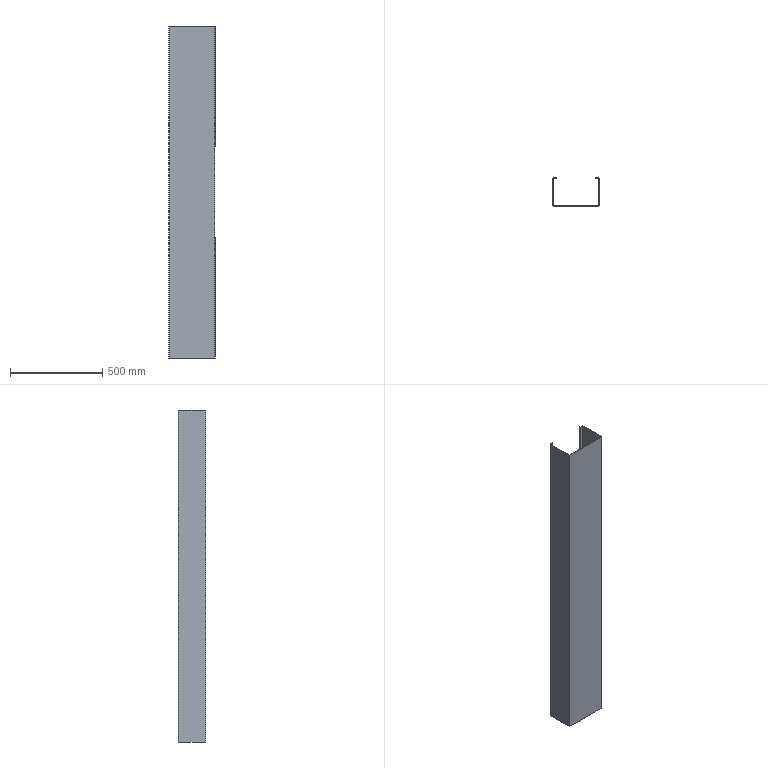Part | STEP file | 750038222 | 1 solid | 36 faces | box 250 x 150 x 1800 mm | volume 1443469 mm3 | plane 25 | cylinder 11 | commonest cylinder face diameters 3 x6 6 x5
STEP:
#1=CARTESIAN_POINT('',(124.598,1.5,248.5));
#2=VERTEX_POINT('',#1);
#3=CARTESIAN_POINT('',(122.,1.5,248.5));
#4=VERTEX_POINT('',#3);
#5=CARTESIAN_POINT('',(125.,1.5,248.5));
#6=DIRECTION('',(-1.,0.,0.));
#7=VECTOR('',#6,1000.);
#8=LINE('',#5,#7);
#9=EDGE_CURVE('',#2,#4,#8,.T.);
#10=ORIENTED_EDGE('',*,*,#9,.F.);
#11=CARTESIAN_POINT('',(124.598,1.5,-248.5));
#12=VERTEX_POINT('',#11);
#13=CARTESIAN_POINT('',(124.598,1.5,900.));
#14=DIRECTION('',(0.,0.,1.));
#15=VECTOR('',#14,1000.);
#16=LINE('',#13,#15);
#17=EDGE_CURVE('',#12,#2,#16,.T.);
#18=ORIENTED_EDGE('',*,*,#17,.F.);
#19=CARTESIAN_POINT('',(122.,1.5,-248.5));
#20=VERTEX_POINT('',#19);
#21=CARTESIAN_POINT('',(125.,1.5,-248.5));
#22=DIRECTION('',(1.,0.,0.));
#23=VECTOR('',#22,1000.);
#24=LINE('',#21,#23);
#25=EDGE_CURVE('',#20,#12,#24,.T.);
#26=ORIENTED_EDGE('',*,*,#25,.F.);
#27=CARTESIAN_POINT('',(122.,1.5,-900.));
#28=VERTEX_POINT('',#27);
#29=CARTESIAN_POINT('',(122.,1.5,900.));
#30=DIRECTION('',(0.,0.,1.));
#31=VECTOR('',#30,1000.);
#32=LINE('',#29,#31);
#33=EDGE_CURVE('',#28,#20,#32,.T.);
#34=ORIENTED_EDGE('',*,*,#33,.F.);
#35=CARTESIAN_POINT('',(-122.,1.5,-900.));
#36=VERTEX_POINT('',#35);
#37=CARTESIAN_POINT('',(125.,1.5,-900.));
#38=DIRECTION('',(1.,0.,0.));
#39=VECTOR('',#38,1000.);
#40=LINE('',#37,#39);
#41=EDGE_CURVE('',#36,#28,#40,.T.);
#42=ORIENTED_EDGE('',*,*,#41,.F.);
#43=CARTESIAN_POINT('',(-122.,1.5,900.));
#44=VERTEX_POINT('',#43);
#45=CARTESIAN_POINT('',(-122.,1.5,900.));
#46=DIRECTION('',(0.,0.,-1.));
#47=VECTOR('',#46,1000.);
#48=LINE('',#45,#47);
#49=EDGE_CURVE('',#44,#36,#48,.T.);
#50=ORIENTED_EDGE('',*,*,#49,.F.);
#51=CARTESIAN_POINT('',(122.,1.5,900.));
#52=VERTEX_POINT('',#51);
#53=CARTESIAN_POINT('',(125.,1.5,900.));
#54=DIRECTION('',(-1.,0.,0.));
#55=VECTOR('',#54,1000.);
#56=LINE('',#53,#55);
#57=EDGE_CURVE('',#52,#44,#56,.T.);
#58=ORIENTED_EDGE('',*,*,#57,.F.);
#59=CARTESIAN_POINT('',(122.,1.5,900.));
#60=DIRECTION('',(0.,0.,1.));
#61=VECTOR('',#60,1000.);
#62=LINE('',#59,#61);
#63=EDGE_CURVE('',#4,#52,#62,.T.);
#64=ORIENTED_EDGE('',*,*,#63,.F.);
#65=EDGE_LOOP('',(#10,#18,#26,#34,#42,#50,#58,#64));
#66=FACE_OUTER_BOUND('',#65,.T.);
#67=CARTESIAN_POINT('',(125.,1.5,900.));
#68=DIRECTION('',(0.,-1.,0.));
#69=DIRECTION('',(0.,0.,-1.));
#70=AXIS2_PLACEMENT_3D('',#67,#68,#69);
#71=PLANE('',#70);
#72=ADVANCED_FACE('',(#66),#71,.F.);
#73=CARTESIAN_POINT('',(123.5,3.,248.5));
#74=VERTEX_POINT('',#73);
#75=CARTESIAN_POINT('',(122.,3.,248.5));
#76=DIRECTION('',(0.,0.,1.));
#77=DIRECTION('',(-1.,0.,0.));
#78=AXIS2_PLACEMENT_3D('',#75,#76,#77);
#79=CIRCLE('',#78,1.5);
#80=EDGE_CURVE('',#4,#74,#79,.T.);
#81=ORIENTED_EDGE('',*,*,#80,.F.);
#82=ORIENTED_EDGE('',*,*,#63,.T.);
#83=CARTESIAN_POINT('',(123.5,3.,900.));
#84=VERTEX_POINT('',#83);
#85=CARTESIAN_POINT('',(122.,3.,900.));
#86=DIRECTION('',(0.,0.,-1.));
#87=DIRECTION('',(-1.,0.,0.));
#88=AXIS2_PLACEMENT_3D('',#85,#86,#87);
#89=CIRCLE('',#88,1.5);
#90=EDGE_CURVE('',#84,#52,#89,.T.);
#91=ORIENTED_EDGE('',*,*,#90,.F.);
#92=CARTESIAN_POINT('',(123.5,3.,900.));
#93=DIRECTION('',(0.,0.,1.));
#94=VECTOR('',#93,1000.);
#95=LINE('',#92,#94);
#96=EDGE_CURVE('',#74,#84,#95,.T.);
#97=ORIENTED_EDGE('',*,*,#96,.F.);
#98=EDGE_LOOP('',(#81,#82,#91,#97));
#99=FACE_OUTER_BOUND('',#98,.T.);
#100=CARTESIAN_POINT('',(122.,3.,900.));
#101=DIRECTION('',(0.,0.,-1.));
#102=DIRECTION('',(-1.,0.,0.));
#103=AXIS2_PLACEMENT_3D('',#100,#101,#102);
#104=CYLINDRICAL_SURFACE('',#103,1.5);
#105=ADVANCED_FACE('',(#99),#104,.F.);
#106=CARTESIAN_POINT('',(125.,147.,248.5));
#107=VERTEX_POINT('',#106);
#108=CARTESIAN_POINT('',(122.,150.,248.5));
#109=VERTEX_POINT('',#108);
#110=CARTESIAN_POINT('',(122.,147.,248.5));
#111=DIRECTION('',(0.,0.,1.));
#112=DIRECTION('',(-1.,0.,0.));
#113=AXIS2_PLACEMENT_3D('',#110,#111,#112);
#114=CIRCLE('',#113,3.);
#115=EDGE_CURVE('',#107,#109,#114,.T.);
#116=ORIENTED_EDGE('',*,*,#115,.F.);
#117=CARTESIAN_POINT('',(125.,3.,248.5));
#118=VERTEX_POINT('',#117);
#119=CARTESIAN_POINT('',(125.,1.5,248.5));
#120=DIRECTION('',(0.,1.,0.));
#121=VECTOR('',#120,1000.);
#122=LINE('',#119,#121);
#123=EDGE_CURVE('',#118,#107,#122,.T.);
#124=ORIENTED_EDGE('',*,*,#123,.F.);
#125=CARTESIAN_POINT('',(122.,3.,248.5));
#126=DIRECTION('',(0.,0.,1.));
#127=DIRECTION('',(-1.,0.,0.));
#128=AXIS2_PLACEMENT_3D('',#125,#126,#127);
#129=CIRCLE('',#128,3.);
#130=EDGE_CURVE('',#2,#118,#129,.T.);
#131=ORIENTED_EDGE('',*,*,#130,.F.);
#132=ORIENTED_EDGE('',*,*,#9,.T.);
#133=ORIENTED_EDGE('',*,*,#80,.T.);
#134=CARTESIAN_POINT('',(123.5,147.,248.5));
#135=VERTEX_POINT('',#134);
#136=CARTESIAN_POINT('',(123.5,1.5,248.5));
#137=DIRECTION('',(0.,-1.,0.));
#138=VECTOR('',#137,1000.);
#139=LINE('',#136,#138);
#140=EDGE_CURVE('',#135,#74,#139,.T.);
#141=ORIENTED_EDGE('',*,*,#140,.F.);
#142=CARTESIAN_POINT('',(122.,148.5,248.5));
#143=VERTEX_POINT('',#142);
#144=CARTESIAN_POINT('',(122.,147.,248.5));
#145=DIRECTION('',(0.,0.,-1.));
#146=DIRECTION('',(-1.,0.,0.));
#147=AXIS2_PLACEMENT_3D('',#144,#145,#146);
#148=CIRCLE('',#147,1.5);
#149=EDGE_CURVE('',#143,#135,#148,.T.);
#150=ORIENTED_EDGE('',*,*,#149,.F.);
#151=CARTESIAN_POINT('',(122.,148.5,248.5));
#152=DIRECTION('',(0.,1.,0.));
#153=VECTOR('',#152,1000.);
#154=LINE('',#151,#153);
#155=EDGE_CURVE('',#143,#109,#154,.T.);
#156=ORIENTED_EDGE('',*,*,#155,.T.);
#157=EDGE_LOOP('',(#116,#124,#131,#132,#133,#141,#150,#156));
#158=FACE_OUTER_BOUND('',#157,.T.);
#159=CARTESIAN_POINT('',(105.,1.5,248.5));
#160=DIRECTION('',(0.,0.,1.));
#161=DIRECTION('',(1.,0.,0.));
#162=AXIS2_PLACEMENT_3D('',#159,#160,#161);
#163=PLANE('',#162);
#164=ADVANCED_FACE('',(#158),#163,.F.);
#165=CARTESIAN_POINT('',(125.,3.,-248.5));
#166=VERTEX_POINT('',#165);
#167=CARTESIAN_POINT('',(122.,3.,-248.5));
#168=DIRECTION('',(0.,0.,-1.));
#169=DIRECTION('',(-1.,0.,0.));
#170=AXIS2_PLACEMENT_3D('',#167,#168,#169);
#171=CIRCLE('',#170,3.);
#172=EDGE_CURVE('',#166,#12,#171,.T.);
#173=ORIENTED_EDGE('',*,*,#172,.T.);
#174=ORIENTED_EDGE('',*,*,#17,.T.);
#175=ORIENTED_EDGE('',*,*,#130,.T.);
#176=CARTESIAN_POINT('',(125.,3.,900.));
#177=VERTEX_POINT('',#176);
#178=CARTESIAN_POINT('',(125.,3.,900.));
#179=DIRECTION('',(0.,0.,1.));
#180=VECTOR('',#179,1000.);
#181=LINE('',#178,#180);
#182=EDGE_CURVE('',#118,#177,#181,.T.);
#183=ORIENTED_EDGE('',*,*,#182,.T.);
#184=CARTESIAN_POINT('',(122.,0.,900.));
#185=VERTEX_POINT('',#184);
#186=CARTESIAN_POINT('',(122.,3.,900.));
#187=DIRECTION('',(0.,0.,-1.));
#188=DIRECTION('',(-1.,0.,0.));
#189=AXIS2_PLACEMENT_3D('',#186,#187,#188);
#190=CIRCLE('',#189,3.);
#191=EDGE_CURVE('',#177,#185,#190,.T.);
#192=ORIENTED_EDGE('',*,*,#191,.T.);
#193=CARTESIAN_POINT('',(122.,0.,-900.));
#194=VERTEX_POINT('',#193);
#195=CARTESIAN_POINT('',(122.,0.,900.));
#196=DIRECTION('',(0.,0.,-1.));
#197=VECTOR('',#196,1000.);
#198=LINE('',#195,#197);
#199=EDGE_CURVE('',#185,#194,#198,.T.);
#200=ORIENTED_EDGE('',*,*,#199,.T.);
#201=CARTESIAN_POINT('',(125.,3.,-900.));
#202=VERTEX_POINT('',#201);
#203=CARTESIAN_POINT('',(122.,3.,-900.));
#204=DIRECTION('',(0.,0.,1.));
#205=DIRECTION('',(-1.,0.,0.));
#206=AXIS2_PLACEMENT_3D('',#203,#204,#205);
#207=CIRCLE('',#206,3.);
#208=EDGE_CURVE('',#194,#202,#207,.T.);
#209=ORIENTED_EDGE('',*,*,#208,.T.);
#210=CARTESIAN_POINT('',(125.,3.,900.));
#211=DIRECTION('',(0.,0.,1.));
#212=VECTOR('',#211,1000.);
#213=LINE('',#210,#212);
#214=EDGE_CURVE('',#202,#166,#213,.T.);
#215=ORIENTED_EDGE('',*,*,#214,.T.);
#216=EDGE_LOOP('',(#173,#174,#175,#183,#192,#200,#209,#215));
#217=FACE_OUTER_BOUND('',#216,.T.);
#218=CARTESIAN_POINT('',(122.,3.,900.));
#219=DIRECTION('',(0.,0.,-1.));
#220=DIRECTION('',(-1.,0.,0.));
#221=AXIS2_PLACEMENT_3D('',#218,#219,#220);
#222=CYLINDRICAL_SURFACE('',#221,3.);
#223=ADVANCED_FACE('',(#217),#222,.T.);
#224=CARTESIAN_POINT('',(122.,148.5,-248.5));
#225=VERTEX_POINT('',#224);
#226=CARTESIAN_POINT('',(122.,150.,-248.5));
#227=VERTEX_POINT('',#226);
#228=CARTESIAN_POINT('',(122.,148.5,-248.5));
#229=DIRECTION('',(0.,1.,0.));
#230=VECTOR('',#229,1000.);
#231=LINE('',#228,#230);
#232=EDGE_CURVE('',#225,#227,#231,.T.);
#233=ORIENTED_EDGE('',*,*,#232,.F.);
#234=CARTESIAN_POINT('',(123.5,147.,-248.5));
#235=VERTEX_POINT('',#234);
#236=CARTESIAN_POINT('',(122.,147.,-248.5));
#237=DIRECTION('',(0.,0.,1.));
#238=DIRECTION('',(-1.,0.,0.));
#239=AXIS2_PLACEMENT_3D('',#236,#237,#238);
#240=CIRCLE('',#239,1.5);
#241=EDGE_CURVE('',#235,#225,#240,.T.);
#242=ORIENTED_EDGE('',*,*,#241,.F.);
#243=CARTESIAN_POINT('',(123.5,3.,-248.5));
#244=VERTEX_POINT('',#243);
#245=CARTESIAN_POINT('',(123.5,1.5,-248.5));
#246=DIRECTION('',(0.,1.,0.));
#247=VECTOR('',#246,1000.);
#248=LINE('',#245,#247);
#249=EDGE_CURVE('',#244,#235,#248,.T.);
#250=ORIENTED_EDGE('',*,*,#249,.F.);
#251=CARTESIAN_POINT('',(122.,3.,-248.5));
#252=DIRECTION('',(0.,0.,1.));
#253=DIRECTION('',(-1.,0.,0.));
#254=AXIS2_PLACEMENT_3D('',#251,#252,#253);
#255=CIRCLE('',#254,1.5);
#256=EDGE_CURVE('',#20,#244,#255,.T.);
#257=ORIENTED_EDGE('',*,*,#256,.F.);
#258=ORIENTED_EDGE('',*,*,#25,.T.);
#259=ORIENTED_EDGE('',*,*,#172,.F.);
#260=CARTESIAN_POINT('',(125.,147.,-248.5));
#261=VERTEX_POINT('',#260);
#262=CARTESIAN_POINT('',(125.,1.5,-248.5));
#263=DIRECTION('',(0.,-1.,0.));
#264=VECTOR('',#263,1000.);
#265=LINE('',#262,#264);
#266=EDGE_CURVE('',#261,#166,#265,.T.);
#267=ORIENTED_EDGE('',*,*,#266,.F.);
#268=CARTESIAN_POINT('',(122.,147.,-248.5));
#269=DIRECTION('',(0.,0.,-1.));
#270=DIRECTION('',(-1.,0.,0.));
#271=AXIS2_PLACEMENT_3D('',#268,#269,#270);
#272=CIRCLE('',#271,3.);
#273=EDGE_CURVE('',#227,#261,#272,.T.);
#274=ORIENTED_EDGE('',*,*,#273,.F.);
#275=EDGE_LOOP('',(#233,#242,#250,#257,#258,#259,#267,#274));
#276=FACE_OUTER_BOUND('',#275,.T.);
#277=CARTESIAN_POINT('',(125.,1.5,-248.5));
#278=DIRECTION('',(0.,0.,-1.));
#279=DIRECTION('',(-1.,0.,0.));
#280=AXIS2_PLACEMENT_3D('',#277,#278,#279);
#281=PLANE('',#280);
#282=ADVANCED_FACE('',(#276),#281,.F.);
#283=ORIENTED_EDGE('',*,*,#256,.T.);
#284=CARTESIAN_POINT('',(123.5,3.,-900.));
#285=VERTEX_POINT('',#284);
#286=CARTESIAN_POINT('',(123.5,3.,900.));
#287=DIRECTION('',(0.,0.,1.));
#288=VECTOR('',#287,1000.);
#289=LINE('',#286,#288);
#290=EDGE_CURVE('',#285,#244,#289,.T.);
#291=ORIENTED_EDGE('',*,*,#290,.F.);
#292=CARTESIAN_POINT('',(122.,3.,-900.));
#293=DIRECTION('',(0.,0.,1.));
#294=DIRECTION('',(-1.,0.,0.));
#295=AXIS2_PLACEMENT_3D('',#292,#293,#294);
#296=CIRCLE('',#295,1.5);
#297=EDGE_CURVE('',#28,#285,#296,.T.);
#298=ORIENTED_EDGE('',*,*,#297,.F.);
#299=ORIENTED_EDGE('',*,*,#33,.T.);
#300=EDGE_LOOP('',(#283,#291,#298,#299));
#301=FACE_OUTER_BOUND('',#300,.T.);
#302=CARTESIAN_POINT('',(122.,3.,900.));
#303=DIRECTION('',(0.,0.,-1.));
#304=DIRECTION('',(-1.,0.,0.));
#305=AXIS2_PLACEMENT_3D('',#302,#303,#304);
#306=CYLINDRICAL_SURFACE('',#305,1.5);
#307=ADVANCED_FACE('',(#301),#306,.F.);
#308=CARTESIAN_POINT('',(105.,148.5,-900.));
#309=VERTEX_POINT('',#308);
#310=CARTESIAN_POINT('',(122.,148.5,-900.));
#311=VERTEX_POINT('',#310);
#312=CARTESIAN_POINT('',(105.,148.5,-900.));
#313=DIRECTION('',(1.,0.,0.));
#314=VECTOR('',#313,1000.);
#315=LINE('',#312,#314);
#316=EDGE_CURVE('',#309,#311,#315,.T.);
#317=ORIENTED_EDGE('',*,*,#316,.F.);
#318=CARTESIAN_POINT('',(105.,150.,-900.));
#319=VERTEX_POINT('',#318);
#320=CARTESIAN_POINT('',(105.,150.,-900.));
#321=DIRECTION('',(0.,1.,0.));
#322=VECTOR('',#321,1000.);
#323=LINE('',#320,#322);
#324=EDGE_CURVE('',#309,#319,#323,.T.);
#325=ORIENTED_EDGE('',*,*,#324,.T.);
#326=CARTESIAN_POINT('',(122.,150.,-900.));
#327=VERTEX_POINT('',#326);
#328=CARTESIAN_POINT('',(105.,150.,-900.));
#329=DIRECTION('',(-1.,0.,0.));
#330=VECTOR('',#329,1000.);
#331=LINE('',#328,#330);
#332=EDGE_CURVE('',#327,#319,#331,.T.);
#333=ORIENTED_EDGE('',*,*,#332,.F.);
#334=CARTESIAN_POINT('',(125.,147.,-900.));
#335=VERTEX_POINT('',#334);
#336=CARTESIAN_POINT('',(122.,147.,-900.));
#337=DIRECTION('',(0.,0.,1.));
#338=DIRECTION('',(-1.,0.,0.));
#339=AXIS2_PLACEMENT_3D('',#336,#337,#338);
#340=CIRCLE('',#339,3.);
#341=EDGE_CURVE('',#335,#327,#340,.T.);
#342=ORIENTED_EDGE('',*,*,#341,.F.);
#343=CARTESIAN_POINT('',(125.,150.,-900.));
#344=DIRECTION('',(0.,1.,0.));
#345=VECTOR('',#344,1000.);
#346=LINE('',#343,#345);
#347=EDGE_CURVE('',#202,#335,#346,.T.);
#348=ORIENTED_EDGE('',*,*,#347,.F.);
#349=ORIENTED_EDGE('',*,*,#208,.F.);
#350=CARTESIAN_POINT('',(-122.,0.,-900.));
#351=VERTEX_POINT('',#350);
#352=CARTESIAN_POINT('',(105.,0.,-900.));
#353=DIRECTION('',(1.,0.,0.));
#354=VECTOR('',#353,1000.);
#355=LINE('',#352,#354);
#356=EDGE_CURVE('',#351,#194,#355,.T.);
#357=ORIENTED_EDGE('',*,*,#356,.F.);
#358=CARTESIAN_POINT('',(-125.,3.,-900.));
#359=VERTEX_POINT('',#358);
#360=CARTESIAN_POINT('',(-122.,3.,-900.));
#361=DIRECTION('',(0.,0.,1.));
#362=DIRECTION('',(-1.,0.,0.));
#363=AXIS2_PLACEMENT_3D('',#360,#361,#362);
#364=CIRCLE('',#363,3.);
#365=EDGE_CURVE('',#359,#351,#364,.T.);
#366=ORIENTED_EDGE('',*,*,#365,.F.);
#367=CARTESIAN_POINT('',(-125.,147.,-900.));
#368=VERTEX_POINT('',#367);
#369=CARTESIAN_POINT('',(-125.,150.,-900.));
#370=DIRECTION('',(0.,-1.,0.));
#371=VECTOR('',#370,1000.);
#372=LINE('',#369,#371);
#373=EDGE_CURVE('',#368,#359,#372,.T.);
#374=ORIENTED_EDGE('',*,*,#373,.F.);
#375=CARTESIAN_POINT('',(-122.,150.,-900.));
#376=VERTEX_POINT('',#375);
#377=CARTESIAN_POINT('',(-122.,147.,-900.));
#378=DIRECTION('',(0.,0.,1.));
#379=DIRECTION('',(-1.,0.,0.));
#380=AXIS2_PLACEMENT_3D('',#377,#378,#379);
#381=CIRCLE('',#380,3.);
#382=EDGE_CURVE('',#376,#368,#381,.T.);
#383=ORIENTED_EDGE('',*,*,#382,.F.);
#384=CARTESIAN_POINT('',(-105.,150.,-900.));
#385=VERTEX_POINT('',#384);
#386=CARTESIAN_POINT('',(105.,150.,-900.));
#387=DIRECTION('',(-1.,0.,0.));
#388=VECTOR('',#387,1000.);
#389=LINE('',#386,#388);
#390=EDGE_CURVE('',#385,#376,#389,.T.);
#391=ORIENTED_EDGE('',*,*,#390,.F.);
#392=CARTESIAN_POINT('',(-105.,148.5,-900.));
#393=VERTEX_POINT('',#392);
#394=CARTESIAN_POINT('',(-105.,150.,-900.));
#395=DIRECTION('',(0.,1.,0.));
#396=VECTOR('',#395,1000.);
#397=LINE('',#394,#396);
#398=EDGE_CURVE('',#393,#385,#397,.T.);
#399=ORIENTED_EDGE('',*,*,#398,.F.);
#400=CARTESIAN_POINT('',(-122.,148.5,-900.));
#401=VERTEX_POINT('',#400);
#402=CARTESIAN_POINT('',(105.,148.5,-900.));
#403=DIRECTION('',(1.,0.,0.));
#404=VECTOR('',#403,1000.);
#405=LINE('',#402,#404);
#406=EDGE_CURVE('',#401,#393,#405,.T.);
#407=ORIENTED_EDGE('',*,*,#406,.F.);
#408=CARTESIAN_POINT('',(-123.5,147.,-900.));
#409=VERTEX_POINT('',#408);
#410=CARTESIAN_POINT('',(-122.,147.,-900.));
#411=DIRECTION('',(0.,0.,-1.));
#412=DIRECTION('',(-1.,0.,0.));
#413=AXIS2_PLACEMENT_3D('',#410,#411,#412);
#414=CIRCLE('',#413,1.5);
#415=EDGE_CURVE('',#409,#401,#414,.T.);
#416=ORIENTED_EDGE('',*,*,#415,.F.);
#417=CARTESIAN_POINT('',(-123.5,3.,-900.));
#418=VERTEX_POINT('',#417);
#419=CARTESIAN_POINT('',(-123.5,150.,-900.));
#420=DIRECTION('',(0.,1.,0.));
#421=VECTOR('',#420,1000.);
#422=LINE('',#419,#421);
#423=EDGE_CURVE('',#418,#409,#422,.T.);
#424=ORIENTED_EDGE('',*,*,#423,.F.);
#425=CARTESIAN_POINT('',(-122.,3.,-900.));
#426=DIRECTION('',(0.,0.,-1.));
#427=DIRECTION('',(-1.,0.,0.));
#428=AXIS2_PLACEMENT_3D('',#425,#426,#427);
#429=CIRCLE('',#428,1.5);
#430=EDGE_CURVE('',#36,#418,#429,.T.);
#431=ORIENTED_EDGE('',*,*,#430,.F.);
#432=ORIENTED_EDGE('',*,*,#41,.T.);
#433=ORIENTED_EDGE('',*,*,#297,.T.);
#434=CARTESIAN_POINT('',(123.5,147.,-900.));
#435=VERTEX_POINT('',#434);
#436=CARTESIAN_POINT('',(123.5,150.,-900.));
#437=DIRECTION('',(0.,-1.,0.));
#438=VECTOR('',#437,1000.);
#439=LINE('',#436,#438);
#440=EDGE_CURVE('',#435,#285,#439,.T.);
#441=ORIENTED_EDGE('',*,*,#440,.F.);
#442=CARTESIAN_POINT('',(122.,147.,-900.));
#443=DIRECTION('',(0.,0.,-1.));
#444=DIRECTION('',(-1.,0.,0.));
#445=AXIS2_PLACEMENT_3D('',#442,#443,#444);
#446=CIRCLE('',#445,1.5);
#447=EDGE_CURVE('',#311,#435,#446,.T.);
#448=ORIENTED_EDGE('',*,*,#447,.F.);
#449=EDGE_LOOP('',(#317,#325,#333,#342,#348,#349,#357,#366,#374,#383,#391,#399,#407,#416,#424,#431,#432,#433,#441,#448));
#450=FACE_OUTER_BOUND('',#449,.T.);
#451=CARTESIAN_POINT('',(105.,150.,-900.));
#452=DIRECTION('',(0.,0.,1.));
#453=DIRECTION('',(1.,0.,0.));
#454=AXIS2_PLACEMENT_3D('',#451,#452,#453);
#455=PLANE('',#454);
#456=ADVANCED_FACE('',(#450),#455,.F.);
#457=CARTESIAN_POINT('',(-123.5,3.,900.));
#458=VERTEX_POINT('',#457);
#459=CARTESIAN_POINT('',(-123.5,3.,900.));
#460=DIRECTION('',(0.,0.,-1.));
#461=VECTOR('',#460,1000.);
#462=LINE('',#459,#461);
#463=EDGE_CURVE('',#458,#418,#462,.T.);
#464=ORIENTED_EDGE('',*,*,#463,.F.);
#465=CARTESIAN_POINT('',(-122.,3.,900.));
#466=DIRECTION('',(0.,0.,-1.));
#467=DIRECTION('',(-1.,0.,0.));
#468=AXIS2_PLACEMENT_3D('',#465,#466,#467);
#469=CIRCLE('',#468,1.5);
#470=EDGE_CURVE('',#44,#458,#469,.T.);
#471=ORIENTED_EDGE('',*,*,#470,.F.);
#472=ORIENTED_EDGE('',*,*,#49,.T.);
#473=ORIENTED_EDGE('',*,*,#430,.T.);
#474=EDGE_LOOP('',(#464,#471,#472,#473));
#475=FACE_OUTER_BOUND('',#474,.T.);
#476=CARTESIAN_POINT('',(-122.,3.,900.));
#477=DIRECTION('',(0.,0.,-1.));
#478=DIRECTION('',(-1.,0.,0.));
#479=AXIS2_PLACEMENT_3D('',#476,#477,#478);
#480=CYLINDRICAL_SURFACE('',#479,1.5);
#481=ADVANCED_FACE('',(#475),#480,.F.);
#482=CARTESIAN_POINT('',(-122.,148.5,900.));
#483=VERTEX_POINT('',#482);
#484=CARTESIAN_POINT('',(-105.,148.5,900.));
#485=VERTEX_POINT('',#484);
#486=CARTESIAN_POINT('',(-125.,148.5,900.));
#487=DIRECTION('',(1.,0.,0.));
#488=VECTOR('',#487,1000.);
#489=LINE('',#486,#488);
#490=EDGE_CURVE('',#483,#485,#489,.T.);
#491=ORIENTED_EDGE('',*,*,#490,.T.);
#492=CARTESIAN_POINT('',(-105.,150.,900.));
#493=VERTEX_POINT('',#492);
#494=CARTESIAN_POINT('',(-105.,150.,900.));
#495=DIRECTION('',(0.,-1.,0.));
#496=VECTOR('',#495,1000.);
#497=LINE('',#494,#496);
#498=EDGE_CURVE('',#493,#485,#497,.T.);
#499=ORIENTED_EDGE('',*,*,#498,.F.);
#500=CARTESIAN_POINT('',(-122.,150.,900.));
#501=VERTEX_POINT('',#500);
#502=CARTESIAN_POINT('',(-125.,150.,900.));
#503=DIRECTION('',(-1.,0.,0.));
#504=VECTOR('',#503,1000.);
#505=LINE('',#502,#504);
#506=EDGE_CURVE('',#493,#501,#505,.T.);
#507=ORIENTED_EDGE('',*,*,#506,.T.);
#508=CARTESIAN_POINT('',(-125.,147.,900.));
#509=VERTEX_POINT('',#508);
#510=CARTESIAN_POINT('',(-122.,147.,900.));
#511=DIRECTION('',(0.,0.,1.));
#512=DIRECTION('',(-1.,0.,0.));
#513=AXIS2_PLACEMENT_3D('',#510,#511,#512);
#514=CIRCLE('',#513,3.);
#515=EDGE_CURVE('',#501,#509,#514,.T.);
#516=ORIENTED_EDGE('',*,*,#515,.T.);
#517=CARTESIAN_POINT('',(-125.,3.,900.));
#518=VERTEX_POINT('',#517);
#519=CARTESIAN_POINT('',(-125.,150.,900.));
#520=DIRECTION('',(0.,-1.,0.));
#521=VECTOR('',#520,1000.);
#522=LINE('',#519,#521);
#523=EDGE_CURVE('',#509,#518,#522,.T.);
#524=ORIENTED_EDGE('',*,*,#523,.T.);
#525=CARTESIAN_POINT('',(-122.,0.,900.));
#526=VERTEX_POINT('',#525);
#527=CARTESIAN_POINT('',(-122.,3.,900.));
#528=DIRECTION('',(0.,0.,1.));
#529=DIRECTION('',(-1.,0.,0.));
#530=AXIS2_PLACEMENT_3D('',#527,#528,#529);
#531=CIRCLE('',#530,3.);
#532=EDGE_CURVE('',#518,#526,#531,.T.);
#533=ORIENTED_EDGE('',*,*,#532,.T.);
#534=CARTESIAN_POINT('',(-125.,0.,900.));
#535=DIRECTION('',(1.,0.,0.));
#536=VECTOR('',#535,1000.);
#537=LINE('',#534,#536);
#538=EDGE_CURVE('',#526,#185,#537,.T.);
#539=ORIENTED_EDGE('',*,*,#538,.T.);
#540=ORIENTED_EDGE('',*,*,#191,.F.);
#541=CARTESIAN_POINT('',(125.,147.,900.));
#542=VERTEX_POINT('',#541);
#543=CARTESIAN_POINT('',(125.,150.,900.));
#544=DIRECTION('',(0.,1.,0.));
#545=VECTOR('',#544,1000.);
#546=LINE('',#543,#545);
#547=EDGE_CURVE('',#177,#542,#546,.T.);
#548=ORIENTED_EDGE('',*,*,#547,.T.);
#549=CARTESIAN_POINT('',(122.,150.,900.));
#550=VERTEX_POINT('',#549);
#551=CARTESIAN_POINT('',(122.,147.,900.));
#552=DIRECTION('',(0.,0.,1.));
#553=DIRECTION('',(-1.,0.,0.));
#554=AXIS2_PLACEMENT_3D('',#551,#552,#553);
#555=CIRCLE('',#554,3.);
#556=EDGE_CURVE('',#542,#550,#555,.T.);
#557=ORIENTED_EDGE('',*,*,#556,.T.);
#558=CARTESIAN_POINT('',(105.,150.,900.));
#559=VERTEX_POINT('',#558);
#560=CARTESIAN_POINT('',(-125.,150.,900.));
#561=DIRECTION('',(-1.,0.,0.));
#562=VECTOR('',#561,1000.);
#563=LINE('',#560,#562);
#564=EDGE_CURVE('',#550,#559,#563,.T.);
#565=ORIENTED_EDGE('',*,*,#564,.T.);
#566=CARTESIAN_POINT('',(105.,148.5,900.));
#567=VERTEX_POINT('',#566);
#568=CARTESIAN_POINT('',(105.,150.,900.));
#569=DIRECTION('',(0.,-1.,0.));
#570=VECTOR('',#569,1000.);
#571=LINE('',#568,#570);
#572=EDGE_CURVE('',#559,#567,#571,.T.);
#573=ORIENTED_EDGE('',*,*,#572,.T.);
#574=CARTESIAN_POINT('',(122.,148.5,900.));
#575=VERTEX_POINT('',#574);
#576=CARTESIAN_POINT('',(-125.,148.5,900.));
#577=DIRECTION('',(1.,0.,0.));
#578=VECTOR('',#577,1000.);
#579=LINE('',#576,#578);
#580=EDGE_CURVE('',#567,#575,#579,.T.);
#581=ORIENTED_EDGE('',*,*,#580,.T.);
#582=CARTESIAN_POINT('',(123.5,147.,900.));
#583=VERTEX_POINT('',#582);
#584=CARTESIAN_POINT('',(122.,147.,900.));
#585=DIRECTION('',(0.,0.,-1.));
#586=DIRECTION('',(-1.,0.,0.));
#587=AXIS2_PLACEMENT_3D('',#584,#585,#586);
#588=CIRCLE('',#587,1.5);
#589=EDGE_CURVE('',#575,#583,#588,.T.);
#590=ORIENTED_EDGE('',*,*,#589,.T.);
#591=CARTESIAN_POINT('',(123.5,150.,900.));
#592=DIRECTION('',(0.,-1.,0.));
#593=VECTOR('',#592,1000.);
#594=LINE('',#591,#593);
#595=EDGE_CURVE('',#583,#84,#594,.T.);
#596=ORIENTED_EDGE('',*,*,#595,.T.);
#597=ORIENTED_EDGE('',*,*,#90,.T.);
#598=ORIENTED_EDGE('',*,*,#57,.T.);
#599=ORIENTED_EDGE('',*,*,#470,.T.);
#600=CARTESIAN_POINT('',(-123.5,147.,900.));
#601=VERTEX_POINT('',#600);
#602=CARTESIAN_POINT('',(-123.5,150.,900.));
#603=DIRECTION('',(0.,1.,0.));
#604=VECTOR('',#603,1000.);
#605=LINE('',#602,#604);
#606=EDGE_CURVE('',#458,#601,#605,.T.);
#607=ORIENTED_EDGE('',*,*,#606,.T.);
#608=CARTESIAN_POINT('',(-122.,147.,900.));
#609=DIRECTION('',(0.,0.,-1.));
#610=DIRECTION('',(-1.,0.,0.));
#611=AXIS2_PLACEMENT_3D('',#608,#609,#610);
#612=CIRCLE('',#611,1.5);
#613=EDGE_CURVE('',#601,#483,#612,.T.);
#614=ORIENTED_EDGE('',*,*,#613,.T.);
#615=EDGE_LOOP('',(#491,#499,#507,#516,#524,#533,#539,#540,#548,#557,#565,#573,#581,#590,#596,#597,#598,#599,#607,#614));
#616=FACE_OUTER_BOUND('',#615,.T.);
#617=CARTESIAN_POINT('',(-125.,150.,900.));
#618=DIRECTION('',(0.,0.,1.));
#619=DIRECTION('',(1.,0.,0.));
#620=AXIS2_PLACEMENT_3D('',#617,#618,#619);
#621=PLANE('',#620);
#622=ADVANCED_FACE('',(#616),#621,.T.);
#623=ORIENTED_EDGE('',*,*,#140,.T.);
#624=ORIENTED_EDGE('',*,*,#96,.T.);
#625=ORIENTED_EDGE('',*,*,#595,.F.);
#626=CARTESIAN_POINT('',(123.5,147.,900.));
#627=DIRECTION('',(0.,0.,1.));
#628=VECTOR('',#627,1000.);
#629=LINE('',#626,#628);
#630=EDGE_CURVE('',#135,#583,#629,.T.);
#631=ORIENTED_EDGE('',*,*,#630,.F.);
#632=EDGE_LOOP('',(#623,#624,#625,#631));
#633=FACE_OUTER_BOUND('',#632,.T.);
#634=CARTESIAN_POINT('',(123.5,150.,900.));
#635=DIRECTION('',(1.,0.,0.));
#636=DIRECTION('',(0.,0.,-1.));
#637=AXIS2_PLACEMENT_3D('',#634,#635,#636);
#638=PLANE('',#637);
#639=ADVANCED_FACE('',(#633),#638,.F.);
#640=ORIENTED_EDGE('',*,*,#556,.F.);
#641=CARTESIAN_POINT('',(125.,147.,900.));
#642=DIRECTION('',(0.,0.,-1.));
#643=VECTOR('',#642,1000.);
#644=LINE('',#641,#643);
#645=EDGE_CURVE('',#542,#107,#644,.T.);
#646=ORIENTED_EDGE('',*,*,#645,.T.);
#647=ORIENTED_EDGE('',*,*,#115,.T.);
#648=CARTESIAN_POINT('',(122.,150.,900.));
#649=DIRECTION('',(0.,0.,1.));
#650=VECTOR('',#649,1000.);
#651=LINE('',#648,#650);
#652=EDGE_CURVE('',#109,#550,#651,.T.);
#653=ORIENTED_EDGE('',*,*,#652,.T.);
#654=EDGE_LOOP('',(#640,#646,#647,#653));
#655=FACE_OUTER_BOUND('',#654,.T.);
#656=CARTESIAN_POINT('',(122.,147.,900.));
#657=DIRECTION('',(0.,0.,-1.));
#658=DIRECTION('',(-1.,0.,0.));
#659=AXIS2_PLACEMENT_3D('',#656,#657,#658);
#660=CYLINDRICAL_SURFACE('',#659,3.);
#661=ADVANCED_FACE('',(#655),#660,.T.);
#662=ORIENTED_EDGE('',*,*,#645,.F.);
#663=ORIENTED_EDGE('',*,*,#547,.F.);
#664=ORIENTED_EDGE('',*,*,#182,.F.);
#665=ORIENTED_EDGE('',*,*,#123,.T.);
#666=EDGE_LOOP('',(#662,#663,#664,#665));
#667=FACE_OUTER_BOUND('',#666,.T.);
#668=CARTESIAN_POINT('',(125.,150.,900.));
#669=DIRECTION('',(1.,0.,0.));
#670=DIRECTION('',(0.,0.,-1.));
#671=AXIS2_PLACEMENT_3D('',#668,#669,#670);
#672=PLANE('',#671);
#673=ADVANCED_FACE('',(#667),#672,.T.);
#674=ORIENTED_EDGE('',*,*,#149,.T.);
#675=ORIENTED_EDGE('',*,*,#630,.T.);
#676=ORIENTED_EDGE('',*,*,#589,.F.);
#677=CARTESIAN_POINT('',(122.,148.5,900.));
#678=DIRECTION('',(0.,0.,1.));
#679=VECTOR('',#678,1000.);
#680=LINE('',#677,#679);
#681=EDGE_CURVE('',#143,#575,#680,.T.);
#682=ORIENTED_EDGE('',*,*,#681,.F.);
#683=EDGE_LOOP('',(#674,#675,#676,#682));
#684=FACE_OUTER_BOUND('',#683,.T.);
#685=CARTESIAN_POINT('',(122.,147.,900.));
#686=DIRECTION('',(0.,0.,-1.));
#687=DIRECTION('',(-1.,0.,0.));
#688=AXIS2_PLACEMENT_3D('',#685,#686,#687);
#689=CYLINDRICAL_SURFACE('',#688,1.5);
#690=ADVANCED_FACE('',(#684),#689,.F.);
#691=ORIENTED_EDGE('',*,*,#347,.T.);
#692=CARTESIAN_POINT('',(125.,147.,900.));
#693=DIRECTION('',(0.,0.,1.));
#694=VECTOR('',#693,1000.);
#695=LINE('',#692,#694);
#696=EDGE_CURVE('',#335,#261,#695,.T.);
#697=ORIENTED_EDGE('',*,*,#696,.T.);
#698=ORIENTED_EDGE('',*,*,#266,.T.);
#699=ORIENTED_EDGE('',*,*,#214,.F.);
#700=EDGE_LOOP('',(#691,#697,#698,#699));
#701=FACE_OUTER_BOUND('',#700,.T.);
#702=CARTESIAN_POINT('',(125.,150.,900.));
#703=DIRECTION('',(1.,0.,0.));
#704=DIRECTION('',(0.,0.,-1.));
#705=AXIS2_PLACEMENT_3D('',#702,#703,#704);
#706=PLANE('',#705);
#707=ADVANCED_FACE('',(#701),#706,.T.);
#708=ORIENTED_EDGE('',*,*,#538,.F.);
#709=CARTESIAN_POINT('',(-122.,0.,900.));
#710=DIRECTION('',(0.,0.,-1.));
#711=VECTOR('',#710,1000.);
#712=LINE('',#709,#711);
#713=EDGE_CURVE('',#526,#351,#712,.T.);
#714=ORIENTED_EDGE('',*,*,#713,.T.);
#715=ORIENTED_EDGE('',*,*,#356,.T.);
#716=ORIENTED_EDGE('',*,*,#199,.F.);
#717=EDGE_LOOP('',(#708,#714,#715,#716));
#718=FACE_OUTER_BOUND('',#717,.T.);
#719=CARTESIAN_POINT('',(125.,0.,900.));
#720=DIRECTION('',(0.,-1.,0.));
#721=DIRECTION('',(0.,0.,-1.));
#722=AXIS2_PLACEMENT_3D('',#719,#720,#721);
#723=PLANE('',#722);
#724=ADVANCED_FACE('',(#718),#723,.T.);
#725=ORIENTED_EDGE('',*,*,#341,.T.);
#726=CARTESIAN_POINT('',(122.,150.,900.));
#727=DIRECTION('',(0.,0.,1.));
#728=VECTOR('',#727,1000.);
#729=LINE('',#726,#728);
#730=EDGE_CURVE('',#327,#227,#729,.T.);
#731=ORIENTED_EDGE('',*,*,#730,.T.);
#732=ORIENTED_EDGE('',*,*,#273,.T.);
#733=ORIENTED_EDGE('',*,*,#696,.F.);
#734=EDGE_LOOP('',(#725,#731,#732,#733));
#735=FACE_OUTER_BOUND('',#734,.T.);
#736=CARTESIAN_POINT('',(122.,147.,900.));
#737=DIRECTION('',(0.,0.,-1.));
#738=DIRECTION('',(-1.,0.,0.));
#739=AXIS2_PLACEMENT_3D('',#736,#737,#738);
#740=CYLINDRICAL_SURFACE('',#739,3.);
#741=ADVANCED_FACE('',(#735),#740,.T.);
#742=ORIENTED_EDGE('',*,*,#241,.T.);
#743=CARTESIAN_POINT('',(122.,148.5,900.));
#744=DIRECTION('',(0.,0.,1.));
#745=VECTOR('',#744,1000.);
#746=LINE('',#743,#745);
#747=EDGE_CURVE('',#311,#225,#746,.T.);
#748=ORIENTED_EDGE('',*,*,#747,.F.);
#749=ORIENTED_EDGE('',*,*,#447,.T.);
#750=CARTESIAN_POINT('',(123.5,147.,900.));
#751=DIRECTION('',(0.,0.,-1.));
#752=VECTOR('',#751,1000.);
#753=LINE('',#750,#752);
#754=EDGE_CURVE('',#235,#435,#753,.T.);
#755=ORIENTED_EDGE('',*,*,#754,.F.);
#756=EDGE_LOOP('',(#742,#748,#749,#755));
#757=FACE_OUTER_BOUND('',#756,.T.);
#758=CARTESIAN_POINT('',(122.,147.,900.));
#759=DIRECTION('',(0.,0.,-1.));
#760=DIRECTION('',(-1.,0.,0.));
#761=AXIS2_PLACEMENT_3D('',#758,#759,#760);
#762=CYLINDRICAL_SURFACE('',#761,1.5);
#763=ADVANCED_FACE('',(#757),#762,.F.);
#764=ORIENTED_EDGE('',*,*,#249,.T.);
#765=ORIENTED_EDGE('',*,*,#754,.T.);
#766=ORIENTED_EDGE('',*,*,#440,.T.);
#767=ORIENTED_EDGE('',*,*,#290,.T.);
#768=EDGE_LOOP('',(#764,#765,#766,#767));
#769=FACE_OUTER_BOUND('',#768,.T.);
#770=CARTESIAN_POINT('',(123.5,150.,900.));
#771=DIRECTION('',(1.,0.,0.));
#772=DIRECTION('',(0.,0.,-1.));
#773=AXIS2_PLACEMENT_3D('',#770,#771,#772);
#774=PLANE('',#773);
#775=ADVANCED_FACE('',(#769),#774,.F.);
#776=CARTESIAN_POINT('',(122.,148.5,-228.5));
#777=VERTEX_POINT('',#776);
#778=CARTESIAN_POINT('',(122.,148.5,900.));
#779=DIRECTION('',(0.,0.,-1.));
#780=VECTOR('',#779,1000.);
#781=LINE('',#778,#780);
#782=EDGE_CURVE('',#777,#225,#781,.T.);
#783=ORIENTED_EDGE('',*,*,#782,.F.);
#784=CARTESIAN_POINT('',(105.,148.5,-228.5));
#785=VERTEX_POINT('',#784);
#786=CARTESIAN_POINT('',(105.,148.5,-228.5));
#787=DIRECTION('',(1.,0.,0.));
#788=VECTOR('',#787,1000.);
#789=LINE('',#786,#788);
#790=EDGE_CURVE('',#785,#777,#789,.T.);
#791=ORIENTED_EDGE('',*,*,#790,.F.);
#792=CARTESIAN_POINT('',(105.,148.5,900.));
#793=DIRECTION('',(0.,0.,1.));
#794=VECTOR('',#793,1000.);
#795=LINE('',#792,#794);
#796=EDGE_CURVE('',#309,#785,#795,.T.);
#797=ORIENTED_EDGE('',*,*,#796,.F.);
#798=ORIENTED_EDGE('',*,*,#316,.T.);
#799=ORIENTED_EDGE('',*,*,#747,.T.);
#800=EDGE_LOOP('',(#783,#791,#797,#798,#799));
#801=FACE_OUTER_BOUND('',#800,.T.);
#802=CARTESIAN_POINT('',(105.,148.5,900.));
#803=DIRECTION('',(0.,1.,0.));
#804=DIRECTION('',(0.,0.,1.));
#805=AXIS2_PLACEMENT_3D('',#802,#803,#804);
#806=PLANE('',#805);
#807=ADVANCED_FACE('',(#801),#806,.F.);
#808=ORIENTED_EDGE('',*,*,#730,.F.);
#809=ORIENTED_EDGE('',*,*,#332,.T.);
#810=CARTESIAN_POINT('',(105.,150.,-228.5));
#811=VERTEX_POINT('',#810);
#812=CARTESIAN_POINT('',(105.,150.,900.));
#813=DIRECTION('',(0.,0.,1.));
#814=VECTOR('',#813,1000.);
#815=LINE('',#812,#814);
#816=EDGE_CURVE('',#319,#811,#815,.T.);
#817=ORIENTED_EDGE('',*,*,#816,.T.);
#818=CARTESIAN_POINT('',(122.,150.,-228.5));
#819=VERTEX_POINT('',#818);
#820=CARTESIAN_POINT('',(105.,150.,-228.5));
#821=DIRECTION('',(1.,0.,0.));
#822=VECTOR('',#821,1000.);
#823=LINE('',#820,#822);
#824=EDGE_CURVE('',#811,#819,#823,.T.);
#825=ORIENTED_EDGE('',*,*,#824,.T.);
#826=CARTESIAN_POINT('',(122.,150.,900.));
#827=DIRECTION('',(0.,0.,-1.));
#828=VECTOR('',#827,1000.);
#829=LINE('',#826,#828);
#830=EDGE_CURVE('',#819,#227,#829,.T.);
#831=ORIENTED_EDGE('',*,*,#830,.T.);
#832=EDGE_LOOP('',(#808,#809,#817,#825,#831));
#833=FACE_OUTER_BOUND('',#832,.T.);
#834=CARTESIAN_POINT('',(105.,150.,900.));
#835=DIRECTION('',(0.,1.,0.));
#836=DIRECTION('',(0.,0.,1.));
#837=AXIS2_PLACEMENT_3D('',#834,#835,#836);
#838=PLANE('',#837);
#839=ADVANCED_FACE('',(#833),#838,.T.);
#840=ORIENTED_EDGE('',*,*,#532,.F.);
#841=CARTESIAN_POINT('',(-125.,3.,900.));
#842=DIRECTION('',(0.,0.,-1.));
#843=VECTOR('',#842,1000.);
#844=LINE('',#841,#843);
#845=EDGE_CURVE('',#518,#359,#844,.T.);
#846=ORIENTED_EDGE('',*,*,#845,.T.);
#847=ORIENTED_EDGE('',*,*,#365,.T.);
#848=ORIENTED_EDGE('',*,*,#713,.F.);
#849=EDGE_LOOP('',(#840,#846,#847,#848));
#850=FACE_OUTER_BOUND('',#849,.T.);
#851=CARTESIAN_POINT('',(-122.,3.,900.));
#852=DIRECTION('',(0.,0.,-1.));
#853=DIRECTION('',(-1.,0.,0.));
#854=AXIS2_PLACEMENT_3D('',#851,#852,#853);
#855=CYLINDRICAL_SURFACE('',#854,3.);
#856=ADVANCED_FACE('',(#850),#855,.T.);
#857=ORIENTED_EDGE('',*,*,#523,.F.);
#858=CARTESIAN_POINT('',(-125.,147.,900.));
#859=DIRECTION('',(0.,0.,-1.));
#860=VECTOR('',#859,1000.);
#861=LINE('',#858,#860);
#862=EDGE_CURVE('',#509,#368,#861,.T.);
#863=ORIENTED_EDGE('',*,*,#862,.T.);
#864=ORIENTED_EDGE('',*,*,#373,.T.);
#865=ORIENTED_EDGE('',*,*,#845,.F.);
#866=EDGE_LOOP('',(#857,#863,#864,#865));
#867=FACE_OUTER_BOUND('',#866,.T.);
#868=CARTESIAN_POINT('',(-125.,0.,900.));
#869=DIRECTION('',(-1.,0.,0.));
#870=DIRECTION('',(0.,0.,1.));
#871=AXIS2_PLACEMENT_3D('',#868,#869,#870);
#872=PLANE('',#871);
#873=ADVANCED_FACE('',(#867),#872,.T.);
#874=ORIENTED_EDGE('',*,*,#515,.F.);
#875=CARTESIAN_POINT('',(-122.,150.,900.));
#876=DIRECTION('',(0.,0.,-1.));
#877=VECTOR('',#876,1000.);
#878=LINE('',#875,#877);
#879=EDGE_CURVE('',#501,#376,#878,.T.);
#880=ORIENTED_EDGE('',*,*,#879,.T.);
#881=ORIENTED_EDGE('',*,*,#382,.T.);
#882=ORIENTED_EDGE('',*,*,#862,.F.);
#883=EDGE_LOOP('',(#874,#880,#881,#882));
#884=FACE_OUTER_BOUND('',#883,.T.);
#885=CARTESIAN_POINT('',(-122.,147.,900.));
#886=DIRECTION('',(0.,0.,-1.));
#887=DIRECTION('',(-1.,0.,0.));
#888=AXIS2_PLACEMENT_3D('',#885,#886,#887);
#889=CYLINDRICAL_SURFACE('',#888,3.);
#890=ADVANCED_FACE('',(#884),#889,.T.);
#891=ORIENTED_EDGE('',*,*,#506,.F.);
#892=CARTESIAN_POINT('',(-105.,150.,900.));
#893=DIRECTION('',(0.,0.,-1.));
#894=VECTOR('',#893,1000.);
#895=LINE('',#892,#894);
#896=EDGE_CURVE('',#493,#385,#895,.T.);
#897=ORIENTED_EDGE('',*,*,#896,.T.);
#898=ORIENTED_EDGE('',*,*,#390,.T.);
#899=ORIENTED_EDGE('',*,*,#879,.F.);
#900=EDGE_LOOP('',(#891,#897,#898,#899));
#901=FACE_OUTER_BOUND('',#900,.T.);
#902=CARTESIAN_POINT('',(-125.,150.,900.));
#903=DIRECTION('',(0.,1.,0.));
#904=DIRECTION('',(0.,0.,1.));
#905=AXIS2_PLACEMENT_3D('',#902,#903,#904);
#906=PLANE('',#905);
#907=ADVANCED_FACE('',(#901),#906,.T.);
#908=CARTESIAN_POINT('',(-105.,148.5,900.));
#909=DIRECTION('',(0.,0.,-1.));
#910=VECTOR('',#909,1000.);
#911=LINE('',#908,#910);
#912=EDGE_CURVE('',#485,#393,#911,.T.);
#913=ORIENTED_EDGE('',*,*,#912,.F.);
#914=ORIENTED_EDGE('',*,*,#490,.F.);
#915=CARTESIAN_POINT('',(-122.,148.5,900.));
#916=DIRECTION('',(0.,0.,1.));
#917=VECTOR('',#916,1000.);
#918=LINE('',#915,#917);
#919=EDGE_CURVE('',#401,#483,#918,.T.);
#920=ORIENTED_EDGE('',*,*,#919,.F.);
#921=ORIENTED_EDGE('',*,*,#406,.T.);
#922=EDGE_LOOP('',(#913,#914,#920,#921));
#923=FACE_OUTER_BOUND('',#922,.T.);
#924=CARTESIAN_POINT('',(-125.,148.5,900.));
#925=DIRECTION('',(0.,1.,0.));
#926=DIRECTION('',(0.,0.,1.));
#927=AXIS2_PLACEMENT_3D('',#924,#925,#926);
#928=PLANE('',#927);
#929=ADVANCED_FACE('',(#923),#928,.F.);
#930=ORIENTED_EDGE('',*,*,#919,.T.);
#931=ORIENTED_EDGE('',*,*,#613,.F.);
#932=CARTESIAN_POINT('',(-123.5,147.,900.));
#933=DIRECTION('',(0.,0.,1.));
#934=VECTOR('',#933,1000.);
#935=LINE('',#932,#934);
#936=EDGE_CURVE('',#409,#601,#935,.T.);
#937=ORIENTED_EDGE('',*,*,#936,.F.);
#938=ORIENTED_EDGE('',*,*,#415,.T.);
#939=EDGE_LOOP('',(#930,#931,#937,#938));
#940=FACE_OUTER_BOUND('',#939,.T.);
#941=CARTESIAN_POINT('',(-122.,147.,900.));
#942=DIRECTION('',(0.,0.,-1.));
#943=DIRECTION('',(-1.,0.,0.));
#944=AXIS2_PLACEMENT_3D('',#941,#942,#943);
#945=CYLINDRICAL_SURFACE('',#944,1.5);
#946=ADVANCED_FACE('',(#940),#945,.F.);
#947=ORIENTED_EDGE('',*,*,#936,.T.);
#948=ORIENTED_EDGE('',*,*,#606,.F.);
#949=ORIENTED_EDGE('',*,*,#463,.T.);
#950=ORIENTED_EDGE('',*,*,#423,.T.);
#951=EDGE_LOOP('',(#947,#948,#949,#950));
#952=FACE_OUTER_BOUND('',#951,.T.);
#953=CARTESIAN_POINT('',(-123.5,0.,900.));
#954=DIRECTION('',(-1.,0.,0.));
#955=DIRECTION('',(0.,0.,1.));
#956=AXIS2_PLACEMENT_3D('',#953,#954,#955);
#957=PLANE('',#956);
#958=ADVANCED_FACE('',(#952),#957,.F.);
#959=CARTESIAN_POINT('',(122.,148.5,228.5));
#960=VERTEX_POINT('',#959);
#961=CARTESIAN_POINT('',(105.,148.5,228.5));
#962=VERTEX_POINT('',#961);
#963=CARTESIAN_POINT('',(105.,148.5,228.5));
#964=DIRECTION('',(-1.,0.,0.));
#965=VECTOR('',#964,1000.);
#966=LINE('',#963,#965);
#967=EDGE_CURVE('',#960,#962,#966,.T.);
#968=ORIENTED_EDGE('',*,*,#967,.F.);
#969=CARTESIAN_POINT('',(122.,148.5,900.));
#970=DIRECTION('',(0.,0.,-1.));
#971=VECTOR('',#970,1000.);
#972=LINE('',#969,#971);
#973=EDGE_CURVE('',#143,#960,#972,.T.);
#974=ORIENTED_EDGE('',*,*,#973,.F.);
#975=ORIENTED_EDGE('',*,*,#681,.T.);
#976=ORIENTED_EDGE('',*,*,#580,.F.);
#977=CARTESIAN_POINT('',(105.,148.5,900.));
#978=DIRECTION('',(0.,0.,1.));
#979=VECTOR('',#978,1000.);
#980=LINE('',#977,#979);
#981=EDGE_CURVE('',#962,#567,#980,.T.);
#982=ORIENTED_EDGE('',*,*,#981,.F.);
#983=EDGE_LOOP('',(#968,#974,#975,#976,#982));
#984=FACE_OUTER_BOUND('',#983,.T.);
#985=CARTESIAN_POINT('',(105.,148.5,900.));
#986=DIRECTION('',(0.,1.,0.));
#987=DIRECTION('',(0.,0.,1.));
#988=AXIS2_PLACEMENT_3D('',#985,#986,#987);
#989=PLANE('',#988);
#990=ADVANCED_FACE('',(#984),#989,.F.);
#991=CARTESIAN_POINT('',(105.,150.,228.5));
#992=VERTEX_POINT('',#991);
#993=CARTESIAN_POINT('',(105.,150.,900.));
#994=DIRECTION('',(0.,0.,1.));
#995=VECTOR('',#994,1000.);
#996=LINE('',#993,#995);
#997=EDGE_CURVE('',#992,#559,#996,.T.);
#998=ORIENTED_EDGE('',*,*,#997,.T.);
#999=ORIENTED_EDGE('',*,*,#564,.F.);
#1000=ORIENTED_EDGE('',*,*,#652,.F.);
#1001=CARTESIAN_POINT('',(122.,150.,228.5));
#1002=VERTEX_POINT('',#1001);
#1003=CARTESIAN_POINT('',(122.,150.,900.));
#1004=DIRECTION('',(0.,0.,-1.));
#1005=VECTOR('',#1004,1000.);
#1006=LINE('',#1003,#1005);
#1007=EDGE_CURVE('',#109,#1002,#1006,.T.);
#1008=ORIENTED_EDGE('',*,*,#1007,.T.);
#1009=CARTESIAN_POINT('',(105.,150.,228.5));
#1010=DIRECTION('',(-1.,0.,0.));
#1011=VECTOR('',#1010,1000.);
#1012=LINE('',#1009,#1011);
#1013=EDGE_CURVE('',#1002,#992,#1012,.T.);
#1014=ORIENTED_EDGE('',*,*,#1013,.T.);
#1015=EDGE_LOOP('',(#998,#999,#1000,#1008,#1014));
#1016=FACE_OUTER_BOUND('',#1015,.T.);
#1017=CARTESIAN_POINT('',(105.,150.,900.));
#1018=DIRECTION('',(0.,1.,0.));
#1019=DIRECTION('',(0.,0.,1.));
#1020=AXIS2_PLACEMENT_3D('',#1017,#1018,#1019);
#1021=PLANE('',#1020);
#1022=ADVANCED_FACE('',(#1016),#1021,.T.);
#1023=ORIENTED_EDGE('',*,*,#782,.T.);
#1024=ORIENTED_EDGE('',*,*,#232,.T.);
#1025=ORIENTED_EDGE('',*,*,#830,.F.);
#1026=CARTESIAN_POINT('',(122.,148.5,-228.5));
#1027=DIRECTION('',(0.,-1.,0.));
#1028=VECTOR('',#1027,1000.);
#1029=LINE('',#1026,#1028);
#1030=EDGE_CURVE('',#819,#777,#1029,.T.);
#1031=ORIENTED_EDGE('',*,*,#1030,.T.);
#1032=EDGE_LOOP('',(#1023,#1024,#1025,#1031));
#1033=FACE_OUTER_BOUND('',#1032,.T.);
#1034=CARTESIAN_POINT('',(122.,148.5,-228.5));
#1035=DIRECTION('',(1.,0.,0.));
#1036=DIRECTION('',(0.,0.,-1.));
#1037=AXIS2_PLACEMENT_3D('',#1034,#1035,#1036);
#1038=PLANE('',#1037);
#1039=ADVANCED_FACE('',(#1033),#1038,.T.);
#1040=ORIENTED_EDGE('',*,*,#790,.T.);
#1041=ORIENTED_EDGE('',*,*,#1030,.F.);
#1042=ORIENTED_EDGE('',*,*,#824,.F.);
#1043=CARTESIAN_POINT('',(105.,148.5,-228.5));
#1044=DIRECTION('',(0.,-1.,0.));
#1045=VECTOR('',#1044,1000.);
#1046=LINE('',#1043,#1045);
#1047=EDGE_CURVE('',#811,#785,#1046,.T.);
#1048=ORIENTED_EDGE('',*,*,#1047,.T.);
#1049=EDGE_LOOP('',(#1040,#1041,#1042,#1048));
#1050=FACE_OUTER_BOUND('',#1049,.T.);
#1051=CARTESIAN_POINT('',(105.,148.5,-228.5));
#1052=DIRECTION('',(0.,0.,1.));
#1053=DIRECTION('',(1.,0.,0.));
#1054=AXIS2_PLACEMENT_3D('',#1051,#1052,#1053);
#1055=PLANE('',#1054);
#1056=ADVANCED_FACE('',(#1050),#1055,.T.);
#1057=ORIENTED_EDGE('',*,*,#1047,.F.);
#1058=ORIENTED_EDGE('',*,*,#816,.F.);
#1059=ORIENTED_EDGE('',*,*,#324,.F.);
#1060=ORIENTED_EDGE('',*,*,#796,.T.);
#1061=EDGE_LOOP('',(#1057,#1058,#1059,#1060));
#1062=FACE_OUTER_BOUND('',#1061,.T.);
#1063=CARTESIAN_POINT('',(105.,150.,900.));
#1064=DIRECTION('',(1.,0.,0.));
#1065=DIRECTION('',(0.,0.,-1.));
#1066=AXIS2_PLACEMENT_3D('',#1063,#1064,#1065);
#1067=PLANE('',#1066);
#1068=ADVANCED_FACE('',(#1062),#1067,.F.);
#1069=ORIENTED_EDGE('',*,*,#398,.T.);
#1070=ORIENTED_EDGE('',*,*,#896,.F.);
#1071=ORIENTED_EDGE('',*,*,#498,.T.);
#1072=ORIENTED_EDGE('',*,*,#912,.T.);
#1073=EDGE_LOOP('',(#1069,#1070,#1071,#1072));
#1074=FACE_OUTER_BOUND('',#1073,.T.);
#1075=CARTESIAN_POINT('',(-105.,150.,900.));
#1076=DIRECTION('',(1.,0.,0.));
#1077=DIRECTION('',(0.,0.,-1.));
#1078=AXIS2_PLACEMENT_3D('',#1075,#1076,#1077);
#1079=PLANE('',#1078);
#1080=ADVANCED_FACE('',(#1074),#1079,.T.);
#1081=CARTESIAN_POINT('',(105.,150.,228.5));
#1082=DIRECTION('',(0.,1.,0.));
#1083=VECTOR('',#1082,1000.);
#1084=LINE('',#1081,#1083);
#1085=EDGE_CURVE('',#962,#992,#1084,.T.);
#1086=ORIENTED_EDGE('',*,*,#1085,.F.);
#1087=ORIENTED_EDGE('',*,*,#981,.T.);
#1088=ORIENTED_EDGE('',*,*,#572,.F.);
#1089=ORIENTED_EDGE('',*,*,#997,.F.);
#1090=EDGE_LOOP('',(#1086,#1087,#1088,#1089));
#1091=FACE_OUTER_BOUND('',#1090,.T.);
#1092=CARTESIAN_POINT('',(105.,150.,900.));
#1093=DIRECTION('',(1.,0.,0.));
#1094=DIRECTION('',(0.,0.,-1.));
#1095=AXIS2_PLACEMENT_3D('',#1092,#1093,#1094);
#1096=PLANE('',#1095);
#1097=ADVANCED_FACE('',(#1091),#1096,.F.);
#1098=CARTESIAN_POINT('',(122.,148.5,228.5));
#1099=DIRECTION('',(0.,1.,0.));
#1100=VECTOR('',#1099,1000.);
#1101=LINE('',#1098,#1100);
#1102=EDGE_CURVE('',#960,#1002,#1101,.T.);
#1103=ORIENTED_EDGE('',*,*,#1102,.F.);
#1104=ORIENTED_EDGE('',*,*,#967,.T.);
#1105=ORIENTED_EDGE('',*,*,#1085,.T.);
#1106=ORIENTED_EDGE('',*,*,#1013,.F.);
#1107=EDGE_LOOP('',(#1103,#1104,#1105,#1106));
#1108=FACE_OUTER_BOUND('',#1107,.T.);
#1109=CARTESIAN_POINT('',(105.,148.5,228.5));
#1110=DIRECTION('',(0.,0.,1.));
#1111=DIRECTION('',(1.,0.,0.));
#1112=AXIS2_PLACEMENT_3D('',#1109,#1110,#1111);
#1113=PLANE('',#1112);
#1114=ADVANCED_FACE('',(#1108),#1113,.F.);
#1115=ORIENTED_EDGE('',*,*,#155,.F.);
#1116=ORIENTED_EDGE('',*,*,#973,.T.);
#1117=ORIENTED_EDGE('',*,*,#1102,.T.);
#1118=ORIENTED_EDGE('',*,*,#1007,.F.);
#1119=EDGE_LOOP('',(#1115,#1116,#1117,#1118));
#1120=FACE_OUTER_BOUND('',#1119,.T.);
#1121=CARTESIAN_POINT('',(122.,148.5,228.5));
#1122=DIRECTION('',(-1.,0.,0.));
#1123=DIRECTION('',(0.,0.,1.));
#1124=AXIS2_PLACEMENT_3D('',#1121,#1122,#1123);
#1125=PLANE('',#1124);
#1126=ADVANCED_FACE('',(#1120),#1125,.F.);
#1127=CLOSED_SHELL('',(#72,#105,#164,#223,#282,#307,#456,#481,#622,#639,#661,#673,#690,#707,#724,#741,#763,#775,#807,#839,#856,#873,#890,#907,#929,#946,#958,#990,#1022,#1039,#1056,#1068,#1080,#1097,#1114,#1126));
#1128=MANIFOLD_SOLID_BREP('',#1127);
#1129=CARTESIAN_POINT('',(0.,0.,0.));
#1130=DIRECTION('',(0.,0.,1.));
#1131=DIRECTION('',(1.,0.,0.));
#1132=AXIS2_PLACEMENT_3D('',#1129,#1130,#1131);
#1133=(LENGTH_UNIT()NAMED_UNIT(*)SI_UNIT(.MILLI.,.METRE.));
#1134=UNCERTAINTY_MEASURE_WITH_UNIT(LENGTH_MEASURE(0.00001),#1133,'','');
#1135=(NAMED_UNIT(*)PLANE_ANGLE_UNIT()SI_UNIT($,.RADIAN.));
#1136=(NAMED_UNIT(*)SI_UNIT($,.STERADIAN.)SOLID_ANGLE_UNIT());
#1137=(GEOMETRIC_REPRESENTATION_CONTEXT(3)GLOBAL_UNCERTAINTY_ASSIGNED_CONTEXT((#1134))GLOBAL_UNIT_ASSIGNED_CONTEXT((#1133,#1135,#1136))REPRESENTATION_CONTEXT('',''));
#1138=ADVANCED_BREP_SHAPE_REPRESENTATION('',(#1128,#1132),#1137);